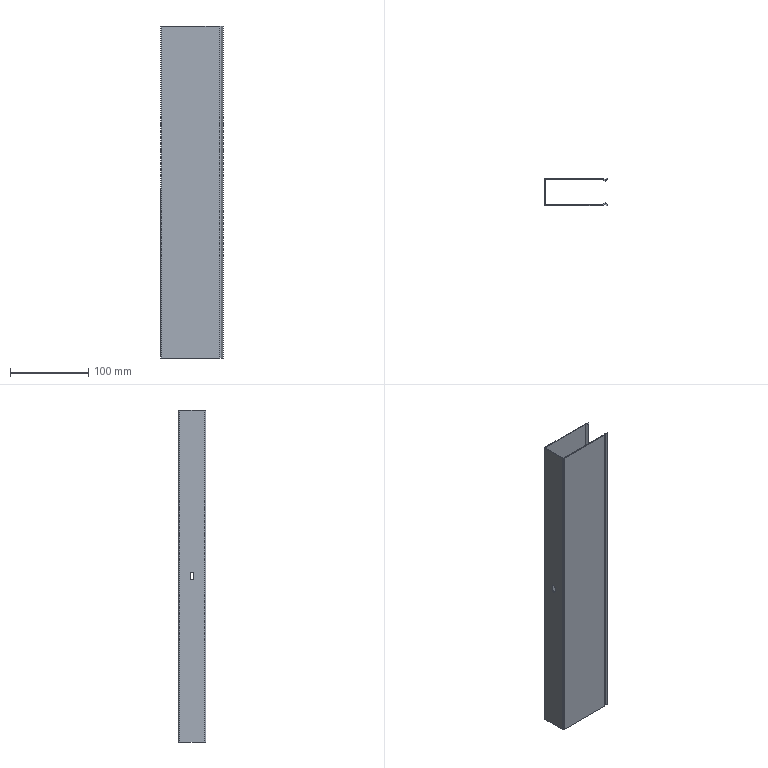Part | STEP file | 35 cable trunking (400) 2 | 1 solid | 27 faces | box 80.625 x 35 x 425 mm | volume 83190 mm3 | plane 20 | cylinder 7 | commonest cylinder face diameters 5 x3 1 x2 3 x2